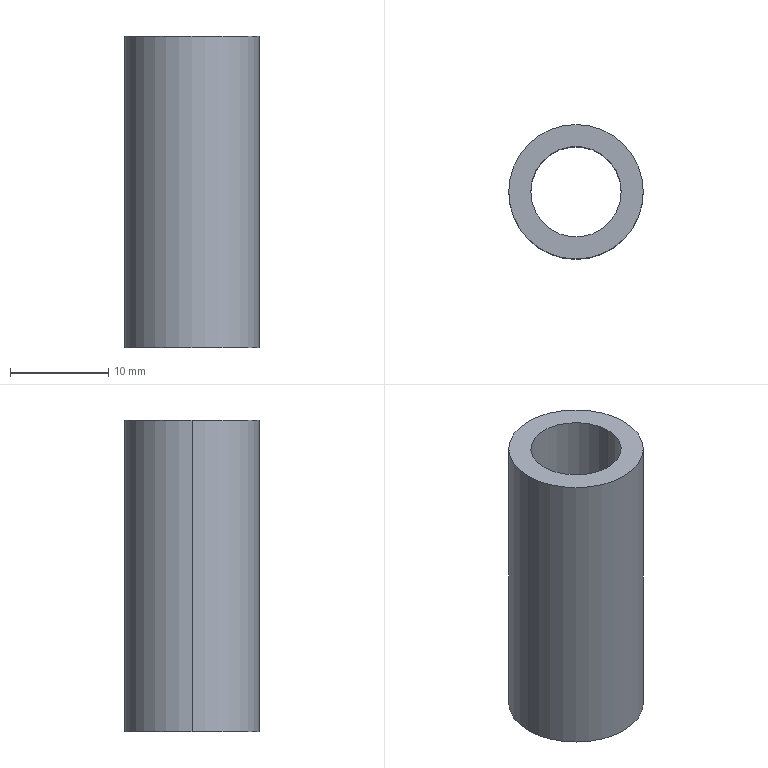Part | SolidWorks | features Extrusion 1 | 1 solid | 6 faces | box 13.7 x 13.7 x 31.75 mm | volume 2561 mm3 | cylinder 4 | plane 2 | commonest cylinder face diameters 9.22 x2 13.7 x2
STEP:
#1=CARTESIAN_POINT('',(-0.1815,0.,0.625));
#2=VERTEX_POINT('',#1);
#3=CARTESIAN_POINT('',(0.1815,0.,0.625));
#4=VERTEX_POINT('',#3);
#5=CARTESIAN_POINT('',(0.,0.,0.625));
#6=DIRECTION('',(0.,0.,1.));
#7=DIRECTION('',(1.,0.,0.));
#8=AXIS2_PLACEMENT_3D('',#5,#6,#7);
#9=CIRCLE('',#8,0.1815);
#10=EDGE_CURVE('',#2,#4,#9,.T.);
#11=ORIENTED_EDGE('',*,*,#10,.T.);
#12=CARTESIAN_POINT('',(0.1815,0.,-0.625));
#13=VERTEX_POINT('',#12);
#14=CARTESIAN_POINT('',(0.1815,0.,0.625));
#15=DIRECTION('',(0.,0.,-1.));
#16=VECTOR('',#15,39.37);
#17=LINE('',#14,#16);
#18=EDGE_CURVE('',#4,#13,#17,.T.);
#19=ORIENTED_EDGE('',*,*,#18,.T.);
#20=CARTESIAN_POINT('',(-0.1815,0.,-0.625));
#21=VERTEX_POINT('',#20);
#22=CARTESIAN_POINT('',(0.,0.,-0.625));
#23=DIRECTION('',(0.,0.,1.));
#24=DIRECTION('',(1.,0.,0.));
#25=AXIS2_PLACEMENT_3D('',#22,#23,#24);
#26=CIRCLE('',#25,0.1815);
#27=EDGE_CURVE('',#21,#13,#26,.T.);
#28=ORIENTED_EDGE('',*,*,#27,.F.);
#29=CARTESIAN_POINT('',(-0.1815,0.,0.625));
#30=DIRECTION('',(0.,0.,-1.));
#31=VECTOR('',#30,39.37);
#32=LINE('',#29,#31);
#33=EDGE_CURVE('',#2,#21,#32,.T.);
#34=ORIENTED_EDGE('',*,*,#33,.F.);
#35=EDGE_LOOP('',(#11,#19,#28,#34));
#36=FACE_OUTER_BOUND('',#35,.T.);
#37=CARTESIAN_POINT('',(0.,0.,0.625));
#38=DIRECTION('',(0.,0.,-1.));
#39=DIRECTION('',(-1.,0.,0.));
#40=AXIS2_PLACEMENT_3D('',#37,#38,#39);
#41=CYLINDRICAL_SURFACE('',#40,0.1815);
#42=ADVANCED_FACE('',(#36),#41,.F.);
#43=CARTESIAN_POINT('',(0.2697,0.,0.625));
#44=VERTEX_POINT('',#43);
#45=CARTESIAN_POINT('',(-0.2697,0.,0.625));
#46=VERTEX_POINT('',#45);
#47=CARTESIAN_POINT('',(0.,0.,0.625));
#48=DIRECTION('',(0.,0.,1.));
#49=DIRECTION('',(1.,0.,0.));
#50=AXIS2_PLACEMENT_3D('',#47,#48,#49);
#51=CIRCLE('',#50,0.2697);
#52=EDGE_CURVE('',#44,#46,#51,.T.);
#53=ORIENTED_EDGE('',*,*,#52,.F.);
#54=CARTESIAN_POINT('',(0.2697,0.,-0.625));
#55=VERTEX_POINT('',#54);
#56=CARTESIAN_POINT('',(0.2697,0.,0.625));
#57=DIRECTION('',(0.,0.,-1.));
#58=VECTOR('',#57,39.37);
#59=LINE('',#56,#58);
#60=EDGE_CURVE('',#44,#55,#59,.T.);
#61=ORIENTED_EDGE('',*,*,#60,.T.);
#62=CARTESIAN_POINT('',(-0.2697,0.,-0.625));
#63=VERTEX_POINT('',#62);
#64=CARTESIAN_POINT('',(0.,0.,-0.625));
#65=DIRECTION('',(0.,0.,1.));
#66=DIRECTION('',(1.,0.,0.));
#67=AXIS2_PLACEMENT_3D('',#64,#65,#66);
#68=CIRCLE('',#67,0.2697);
#69=EDGE_CURVE('',#55,#63,#68,.T.);
#70=ORIENTED_EDGE('',*,*,#69,.T.);
#71=CARTESIAN_POINT('',(-0.2697,0.,0.625));
#72=DIRECTION('',(0.,0.,-1.));
#73=VECTOR('',#72,39.37);
#74=LINE('',#71,#73);
#75=EDGE_CURVE('',#46,#63,#74,.T.);
#76=ORIENTED_EDGE('',*,*,#75,.F.);
#77=EDGE_LOOP('',(#53,#61,#70,#76));
#78=FACE_OUTER_BOUND('',#77,.T.);
#79=CARTESIAN_POINT('',(0.,0.,0.625));
#80=DIRECTION('',(0.,0.,-1.));
#81=DIRECTION('',(-1.,0.,0.));
#82=AXIS2_PLACEMENT_3D('',#79,#80,#81);
#83=CYLINDRICAL_SURFACE('',#82,0.2697);
#84=ADVANCED_FACE('',(#78),#83,.T.);
#85=CARTESIAN_POINT('',(0.,0.,0.625));
#86=DIRECTION('',(0.,0.,1.));
#87=DIRECTION('',(1.,0.,0.));
#88=AXIS2_PLACEMENT_3D('',#85,#86,#87);
#89=CIRCLE('',#88,0.2697);
#90=EDGE_CURVE('',#46,#44,#89,.T.);
#91=ORIENTED_EDGE('',*,*,#90,.T.);
#92=ORIENTED_EDGE('',*,*,#52,.T.);
#93=EDGE_LOOP('',(#91,#92));
#94=FACE_OUTER_BOUND('',#93,.T.);
#95=ORIENTED_EDGE('',*,*,#10,.F.);
#96=CARTESIAN_POINT('',(0.,0.,0.625));
#97=DIRECTION('',(0.,0.,1.));
#98=DIRECTION('',(1.,0.,0.));
#99=AXIS2_PLACEMENT_3D('',#96,#97,#98);
#100=CIRCLE('',#99,0.1815);
#101=EDGE_CURVE('',#4,#2,#100,.T.);
#102=ORIENTED_EDGE('',*,*,#101,.F.);
#103=EDGE_LOOP('',(#95,#102));
#104=FACE_BOUND('',#103,.T.);
#105=CARTESIAN_POINT('',(0.,0.,0.625));
#106=DIRECTION('',(0.,0.,1.));
#107=DIRECTION('',(1.,0.,0.));
#108=AXIS2_PLACEMENT_3D('',#105,#106,#107);
#109=PLANE('',#108);
#110=ADVANCED_FACE('',(#94,#104),#109,.T.);
#111=CARTESIAN_POINT('',(0.,0.,-0.625));
#112=DIRECTION('',(0.,0.,1.));
#113=DIRECTION('',(1.,0.,0.));
#114=AXIS2_PLACEMENT_3D('',#111,#112,#113);
#115=CIRCLE('',#114,0.2697);
#116=EDGE_CURVE('',#63,#55,#115,.T.);
#117=ORIENTED_EDGE('',*,*,#116,.F.);
#118=ORIENTED_EDGE('',*,*,#69,.F.);
#119=EDGE_LOOP('',(#117,#118));
#120=FACE_OUTER_BOUND('',#119,.T.);
#121=ORIENTED_EDGE('',*,*,#27,.T.);
#122=CARTESIAN_POINT('',(0.,0.,-0.625));
#123=DIRECTION('',(0.,0.,1.));
#124=DIRECTION('',(1.,0.,0.));
#125=AXIS2_PLACEMENT_3D('',#122,#123,#124);
#126=CIRCLE('',#125,0.1815);
#127=EDGE_CURVE('',#13,#21,#126,.T.);
#128=ORIENTED_EDGE('',*,*,#127,.T.);
#129=EDGE_LOOP('',(#121,#128));
#130=FACE_BOUND('',#129,.T.);
#131=CARTESIAN_POINT('',(0.,0.,-0.625));
#132=DIRECTION('',(0.,0.,1.));
#133=DIRECTION('',(1.,0.,0.));
#134=AXIS2_PLACEMENT_3D('',#131,#132,#133);
#135=PLANE('',#134);
#136=ADVANCED_FACE('',(#120,#130),#135,.F.);
#137=ORIENTED_EDGE('',*,*,#60,.F.);
#138=ORIENTED_EDGE('',*,*,#90,.F.);
#139=ORIENTED_EDGE('',*,*,#75,.T.);
#140=ORIENTED_EDGE('',*,*,#116,.T.);
#141=EDGE_LOOP('',(#137,#138,#139,#140));
#142=FACE_OUTER_BOUND('',#141,.T.);
#143=CARTESIAN_POINT('',(0.,0.,0.625));
#144=DIRECTION('',(0.,0.,-1.));
#145=DIRECTION('',(-1.,0.,0.));
#146=AXIS2_PLACEMENT_3D('',#143,#144,#145);
#147=CYLINDRICAL_SURFACE('',#146,0.2697);
#148=ADVANCED_FACE('',(#142),#147,.T.);
#149=ORIENTED_EDGE('',*,*,#18,.F.);
#150=ORIENTED_EDGE('',*,*,#101,.T.);
#151=ORIENTED_EDGE('',*,*,#33,.T.);
#152=ORIENTED_EDGE('',*,*,#127,.F.);
#153=EDGE_LOOP('',(#149,#150,#151,#152));
#154=FACE_OUTER_BOUND('',#153,.T.);
#155=CARTESIAN_POINT('',(0.,0.,0.625));
#156=DIRECTION('',(0.,0.,-1.));
#157=DIRECTION('',(-1.,0.,0.));
#158=AXIS2_PLACEMENT_3D('',#155,#156,#157);
#159=CYLINDRICAL_SURFACE('',#158,0.1815);
#160=ADVANCED_FACE('',(#154),#159,.F.);
#161=CLOSED_SHELL('',(#42,#84,#110,#136,#148,#160));
#162=MANIFOLD_SOLID_BREP('',#161);
#163=CARTESIAN_POINT('',(0.,0.,0.));
#164=DIRECTION('',(0.,0.,1.));
#165=DIRECTION('',(1.,0.,0.));
#166=AXIS2_PLACEMENT_3D('',#163,#164,#165);
#167=(LENGTH_UNIT()NAMED_UNIT(*)SI_UNIT($,.METRE.));
#168=LENGTH_MEASURE_WITH_UNIT(LENGTH_MEASURE(0.0254),#167);
#169=DIMENSIONAL_EXPONENTS(1.,0.,0.,0.,0.,0.,0.);
#170=(CONVERSION_BASED_UNIT('INCH',#168)LENGTH_UNIT()NAMED_UNIT(#169));
#171=UNCERTAINTY_MEASURE_WITH_UNIT(LENGTH_MEASURE(0.00001),#170,'','');
#172=(NAMED_UNIT(*)PLANE_ANGLE_UNIT()SI_UNIT($,.RADIAN.));
#173=(NAMED_UNIT(*)SI_UNIT($,.STERADIAN.)SOLID_ANGLE_UNIT());
#174=(GEOMETRIC_REPRESENTATION_CONTEXT(3)GLOBAL_UNCERTAINTY_ASSIGNED_CONTEXT((#171))GLOBAL_UNIT_ASSIGNED_CONTEXT((#170,#172,#173))REPRESENTATION_CONTEXT('',''));
#175=ADVANCED_BREP_SHAPE_REPRESENTATION('',(#162,#166),#174);